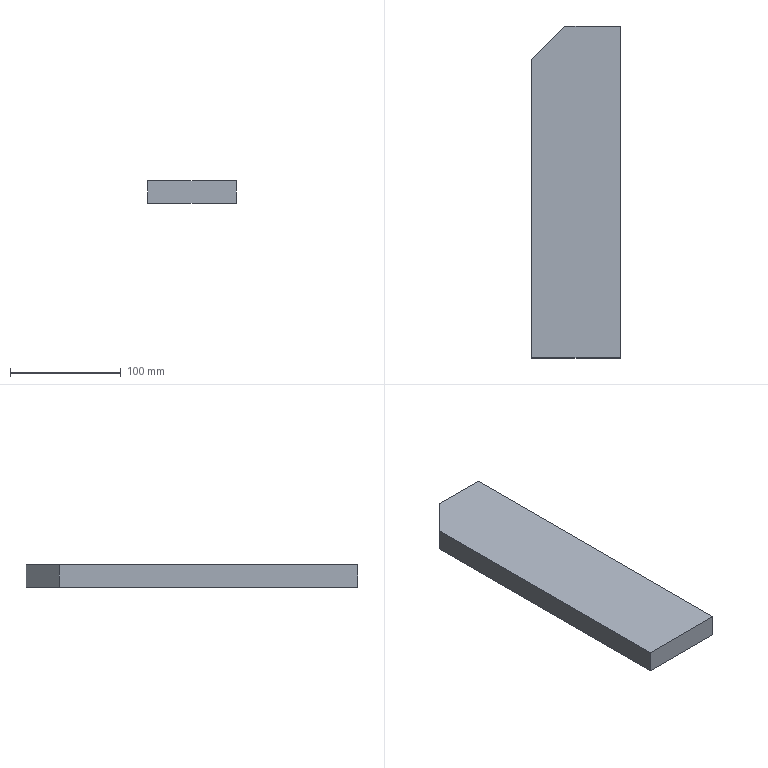Part | SolidWorks | features Extrusion 1 | 1 solid | 7 faces | box 80 x 300 x 20 mm | volume 471000 mm3 | plane 7
STEP:
#1=CARTESIAN_POINT('',(0.,0.,0.));
#2=VERTEX_POINT('',#1);
#3=CARTESIAN_POINT('',(0.,300.,0.));
#4=VERTEX_POINT('',#3);
#5=CARTESIAN_POINT('',(0.,0.,0.));
#6=DIRECTION('',(0.,1.,0.));
#7=VECTOR('',#6,1000.);
#8=LINE('',#5,#7);
#9=EDGE_CURVE('',#2,#4,#8,.T.);
#10=ORIENTED_EDGE('',*,*,#9,.T.);
#11=CARTESIAN_POINT('',(0.,300.,20.));
#12=VERTEX_POINT('',#11);
#13=CARTESIAN_POINT('',(0.,300.,20.));
#14=DIRECTION('',(0.,0.,-1.));
#15=VECTOR('',#14,1000.);
#16=LINE('',#13,#15);
#17=EDGE_CURVE('',#12,#4,#16,.T.);
#18=ORIENTED_EDGE('',*,*,#17,.F.);
#19=CARTESIAN_POINT('',(0.,0.,20.));
#20=VERTEX_POINT('',#19);
#21=CARTESIAN_POINT('',(0.,0.,20.));
#22=DIRECTION('',(0.,1.,0.));
#23=VECTOR('',#22,1000.);
#24=LINE('',#21,#23);
#25=EDGE_CURVE('',#20,#12,#24,.T.);
#26=ORIENTED_EDGE('',*,*,#25,.F.);
#27=CARTESIAN_POINT('',(0.,0.,20.));
#28=DIRECTION('',(0.,0.,-1.));
#29=VECTOR('',#28,1000.);
#30=LINE('',#27,#29);
#31=EDGE_CURVE('',#20,#2,#30,.T.);
#32=ORIENTED_EDGE('',*,*,#31,.T.);
#33=EDGE_LOOP('',(#10,#18,#26,#32));
#34=FACE_OUTER_BOUND('',#33,.T.);
#35=CARTESIAN_POINT('',(0.,0.,20.));
#36=DIRECTION('',(-1.,0.,0.));
#37=DIRECTION('',(0.,0.,1.));
#38=AXIS2_PLACEMENT_3D('',#35,#36,#37);
#39=PLANE('',#38);
#40=ADVANCED_FACE('',(#34),#39,.F.);
#41=CARTESIAN_POINT('',(-50.,300.,0.));
#42=VERTEX_POINT('',#41);
#43=CARTESIAN_POINT('',(0.,300.,0.));
#44=DIRECTION('',(-1.,0.,0.));
#45=VECTOR('',#44,1000.);
#46=LINE('',#43,#45);
#47=EDGE_CURVE('',#4,#42,#46,.T.);
#48=ORIENTED_EDGE('',*,*,#47,.T.);
#49=CARTESIAN_POINT('',(-50.,300.,20.));
#50=VERTEX_POINT('',#49);
#51=CARTESIAN_POINT('',(-50.,300.,20.));
#52=DIRECTION('',(0.,0.,-1.));
#53=VECTOR('',#52,1000.);
#54=LINE('',#51,#53);
#55=EDGE_CURVE('',#50,#42,#54,.T.);
#56=ORIENTED_EDGE('',*,*,#55,.F.);
#57=CARTESIAN_POINT('',(0.,300.,20.));
#58=DIRECTION('',(-1.,0.,0.));
#59=VECTOR('',#58,1000.);
#60=LINE('',#57,#59);
#61=EDGE_CURVE('',#12,#50,#60,.T.);
#62=ORIENTED_EDGE('',*,*,#61,.F.);
#63=ORIENTED_EDGE('',*,*,#17,.T.);
#64=EDGE_LOOP('',(#48,#56,#62,#63));
#65=FACE_OUTER_BOUND('',#64,.T.);
#66=CARTESIAN_POINT('',(0.,300.,20.));
#67=DIRECTION('',(0.,-1.,0.));
#68=DIRECTION('',(0.,0.,-1.));
#69=AXIS2_PLACEMENT_3D('',#66,#67,#68);
#70=PLANE('',#69);
#71=ADVANCED_FACE('',(#65),#70,.F.);
#72=CARTESIAN_POINT('',(-80.,270.,0.));
#73=VERTEX_POINT('',#72);
#74=CARTESIAN_POINT('',(-50.,300.,0.));
#75=DIRECTION('',(-0.7071,-0.7071,0.));
#76=VECTOR('',#75,1000.);
#77=LINE('',#74,#76);
#78=EDGE_CURVE('',#42,#73,#77,.T.);
#79=ORIENTED_EDGE('',*,*,#78,.T.);
#80=CARTESIAN_POINT('',(-80.,270.,20.));
#81=VERTEX_POINT('',#80);
#82=CARTESIAN_POINT('',(-80.,270.,20.));
#83=DIRECTION('',(0.,0.,-1.));
#84=VECTOR('',#83,1000.);
#85=LINE('',#82,#84);
#86=EDGE_CURVE('',#81,#73,#85,.T.);
#87=ORIENTED_EDGE('',*,*,#86,.F.);
#88=CARTESIAN_POINT('',(-50.,300.,20.));
#89=DIRECTION('',(-0.7071,-0.7071,0.));
#90=VECTOR('',#89,1000.);
#91=LINE('',#88,#90);
#92=EDGE_CURVE('',#50,#81,#91,.T.);
#93=ORIENTED_EDGE('',*,*,#92,.F.);
#94=ORIENTED_EDGE('',*,*,#55,.T.);
#95=EDGE_LOOP('',(#79,#87,#93,#94));
#96=FACE_OUTER_BOUND('',#95,.T.);
#97=CARTESIAN_POINT('',(-50.,300.,20.));
#98=DIRECTION('',(0.7071,-0.7071,0.));
#99=DIRECTION('',(0.7071,0.7071,0.));
#100=AXIS2_PLACEMENT_3D('',#97,#98,#99);
#101=PLANE('',#100);
#102=ADVANCED_FACE('',(#96),#101,.F.);
#103=CARTESIAN_POINT('',(-80.,0.,0.));
#104=VERTEX_POINT('',#103);
#105=CARTESIAN_POINT('',(-80.,0.,0.));
#106=DIRECTION('',(0.,-1.,0.));
#107=VECTOR('',#106,1000.);
#108=LINE('',#105,#107);
#109=EDGE_CURVE('',#73,#104,#108,.T.);
#110=ORIENTED_EDGE('',*,*,#109,.T.);
#111=CARTESIAN_POINT('',(-80.,0.,20.));
#112=VERTEX_POINT('',#111);
#113=CARTESIAN_POINT('',(-80.,0.,20.));
#114=DIRECTION('',(0.,0.,-1.));
#115=VECTOR('',#114,1000.);
#116=LINE('',#113,#115);
#117=EDGE_CURVE('',#112,#104,#116,.T.);
#118=ORIENTED_EDGE('',*,*,#117,.F.);
#119=CARTESIAN_POINT('',(-80.,0.,20.));
#120=DIRECTION('',(0.,-1.,0.));
#121=VECTOR('',#120,1000.);
#122=LINE('',#119,#121);
#123=EDGE_CURVE('',#81,#112,#122,.T.);
#124=ORIENTED_EDGE('',*,*,#123,.F.);
#125=ORIENTED_EDGE('',*,*,#86,.T.);
#126=EDGE_LOOP('',(#110,#118,#124,#125));
#127=FACE_OUTER_BOUND('',#126,.T.);
#128=CARTESIAN_POINT('',(-80.,0.,20.));
#129=DIRECTION('',(1.,0.,0.));
#130=DIRECTION('',(0.,0.,-1.));
#131=AXIS2_PLACEMENT_3D('',#128,#129,#130);
#132=PLANE('',#131);
#133=ADVANCED_FACE('',(#127),#132,.F.);
#134=CARTESIAN_POINT('',(0.,0.,0.));
#135=DIRECTION('',(1.,0.,0.));
#136=VECTOR('',#135,1000.);
#137=LINE('',#134,#136);
#138=EDGE_CURVE('',#104,#2,#137,.T.);
#139=ORIENTED_EDGE('',*,*,#138,.T.);
#140=ORIENTED_EDGE('',*,*,#31,.F.);
#141=CARTESIAN_POINT('',(0.,0.,20.));
#142=DIRECTION('',(1.,0.,0.));
#143=VECTOR('',#142,1000.);
#144=LINE('',#141,#143);
#145=EDGE_CURVE('',#112,#20,#144,.T.);
#146=ORIENTED_EDGE('',*,*,#145,.F.);
#147=ORIENTED_EDGE('',*,*,#117,.T.);
#148=EDGE_LOOP('',(#139,#140,#146,#147));
#149=FACE_OUTER_BOUND('',#148,.T.);
#150=CARTESIAN_POINT('',(0.,0.,20.));
#151=DIRECTION('',(0.,1.,0.));
#152=DIRECTION('',(0.,0.,1.));
#153=AXIS2_PLACEMENT_3D('',#150,#151,#152);
#154=PLANE('',#153);
#155=ADVANCED_FACE('',(#149),#154,.F.);
#156=ORIENTED_EDGE('',*,*,#25,.T.);
#157=ORIENTED_EDGE('',*,*,#61,.T.);
#158=ORIENTED_EDGE('',*,*,#92,.T.);
#159=ORIENTED_EDGE('',*,*,#123,.T.);
#160=ORIENTED_EDGE('',*,*,#145,.T.);
#161=EDGE_LOOP('',(#156,#157,#158,#159,#160));
#162=FACE_OUTER_BOUND('',#161,.T.);
#163=CARTESIAN_POINT('',(0.,0.,20.));
#164=DIRECTION('',(0.,0.,1.));
#165=DIRECTION('',(1.,0.,0.));
#166=AXIS2_PLACEMENT_3D('',#163,#164,#165);
#167=PLANE('',#166);
#168=ADVANCED_FACE('',(#162),#167,.T.);
#169=ORIENTED_EDGE('',*,*,#9,.F.);
#170=ORIENTED_EDGE('',*,*,#138,.F.);
#171=ORIENTED_EDGE('',*,*,#109,.F.);
#172=ORIENTED_EDGE('',*,*,#78,.F.);
#173=ORIENTED_EDGE('',*,*,#47,.F.);
#174=EDGE_LOOP('',(#169,#170,#171,#172,#173));
#175=FACE_OUTER_BOUND('',#174,.T.);
#176=CARTESIAN_POINT('',(0.,0.,0.));
#177=DIRECTION('',(0.,0.,1.));
#178=DIRECTION('',(1.,0.,0.));
#179=AXIS2_PLACEMENT_3D('',#176,#177,#178);
#180=PLANE('',#179);
#181=ADVANCED_FACE('',(#175),#180,.F.);
#182=CLOSED_SHELL('',(#40,#71,#102,#133,#155,#168,#181));
#183=MANIFOLD_SOLID_BREP('',#182);
#184=CARTESIAN_POINT('',(0.,0.,0.));
#185=DIRECTION('',(0.,0.,1.));
#186=DIRECTION('',(1.,0.,0.));
#187=AXIS2_PLACEMENT_3D('',#184,#185,#186);
#188=(LENGTH_UNIT()NAMED_UNIT(*)SI_UNIT(.MILLI.,.METRE.));
#189=UNCERTAINTY_MEASURE_WITH_UNIT(LENGTH_MEASURE(0.00001),#188,'','');
#190=(NAMED_UNIT(*)PLANE_ANGLE_UNIT()SI_UNIT($,.RADIAN.));
#191=(NAMED_UNIT(*)SI_UNIT($,.STERADIAN.)SOLID_ANGLE_UNIT());
#192=(GEOMETRIC_REPRESENTATION_CONTEXT(3)GLOBAL_UNCERTAINTY_ASSIGNED_CONTEXT((#189))GLOBAL_UNIT_ASSIGNED_CONTEXT((#188,#190,#191))REPRESENTATION_CONTEXT('',''));
#193=ADVANCED_BREP_SHAPE_REPRESENTATION('',(#183,#187),#192);